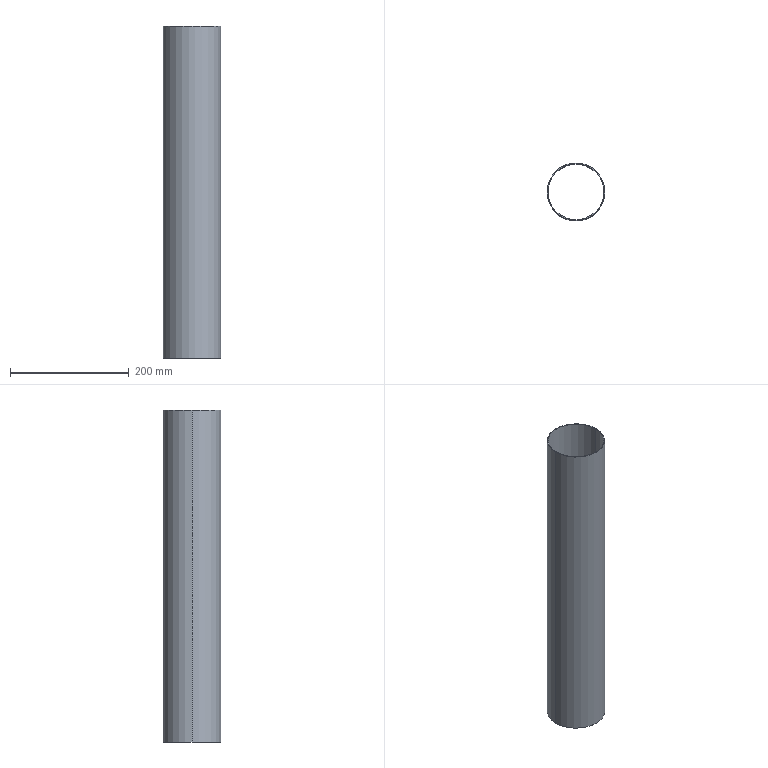Part | SolidWorks | features Extrusion 1 | 1 solid | 6 faces | box 97 x 97 x 558.5 mm | volume 201706 mm3 | cylinder 4 | plane 2 | commonest cylinder face diameters 94.6 x2 97 x2
STEP:
#1=CARTESIAN_POINT('',(-47.3,0.,558.5));
#2=VERTEX_POINT('',#1);
#3=CARTESIAN_POINT('',(47.3,0.,558.5));
#4=VERTEX_POINT('',#3);
#5=CARTESIAN_POINT('',(0.,0.,558.5));
#6=DIRECTION('',(0.,0.,1.));
#7=DIRECTION('',(1.,0.,0.));
#8=AXIS2_PLACEMENT_3D('',#5,#6,#7);
#9=CIRCLE('',#8,47.3);
#10=EDGE_CURVE('',#2,#4,#9,.T.);
#11=ORIENTED_EDGE('',*,*,#10,.T.);
#12=CARTESIAN_POINT('',(47.3,0.,0.));
#13=VERTEX_POINT('',#12);
#14=CARTESIAN_POINT('',(47.3,0.,558.5));
#15=DIRECTION('',(0.,0.,-1.));
#16=VECTOR('',#15,1000.);
#17=LINE('',#14,#16);
#18=EDGE_CURVE('',#4,#13,#17,.T.);
#19=ORIENTED_EDGE('',*,*,#18,.T.);
#20=CARTESIAN_POINT('',(-47.3,0.,0.));
#21=VERTEX_POINT('',#20);
#22=CARTESIAN_POINT('',(0.,0.,0.));
#23=DIRECTION('',(0.,0.,1.));
#24=DIRECTION('',(1.,0.,0.));
#25=AXIS2_PLACEMENT_3D('',#22,#23,#24);
#26=CIRCLE('',#25,47.3);
#27=EDGE_CURVE('',#21,#13,#26,.T.);
#28=ORIENTED_EDGE('',*,*,#27,.F.);
#29=CARTESIAN_POINT('',(-47.3,0.,558.5));
#30=DIRECTION('',(0.,0.,-1.));
#31=VECTOR('',#30,1000.);
#32=LINE('',#29,#31);
#33=EDGE_CURVE('',#2,#21,#32,.T.);
#34=ORIENTED_EDGE('',*,*,#33,.F.);
#35=EDGE_LOOP('',(#11,#19,#28,#34));
#36=FACE_OUTER_BOUND('',#35,.T.);
#37=CARTESIAN_POINT('',(0.,0.,558.5));
#38=DIRECTION('',(0.,0.,-1.));
#39=DIRECTION('',(-1.,0.,0.));
#40=AXIS2_PLACEMENT_3D('',#37,#38,#39);
#41=CYLINDRICAL_SURFACE('',#40,47.3);
#42=ADVANCED_FACE('',(#36),#41,.F.);
#43=CARTESIAN_POINT('',(48.5,0.,558.5));
#44=VERTEX_POINT('',#43);
#45=CARTESIAN_POINT('',(-48.5,0.,558.5));
#46=VERTEX_POINT('',#45);
#47=CARTESIAN_POINT('',(0.,0.,558.5));
#48=DIRECTION('',(0.,0.,1.));
#49=DIRECTION('',(1.,0.,0.));
#50=AXIS2_PLACEMENT_3D('',#47,#48,#49);
#51=CIRCLE('',#50,48.5);
#52=EDGE_CURVE('',#44,#46,#51,.T.);
#53=ORIENTED_EDGE('',*,*,#52,.F.);
#54=CARTESIAN_POINT('',(48.5,0.,0.));
#55=VERTEX_POINT('',#54);
#56=CARTESIAN_POINT('',(48.5,0.,558.5));
#57=DIRECTION('',(0.,0.,-1.));
#58=VECTOR('',#57,1000.);
#59=LINE('',#56,#58);
#60=EDGE_CURVE('',#44,#55,#59,.T.);
#61=ORIENTED_EDGE('',*,*,#60,.T.);
#62=CARTESIAN_POINT('',(-48.5,0.,0.));
#63=VERTEX_POINT('',#62);
#64=CARTESIAN_POINT('',(0.,0.,0.));
#65=DIRECTION('',(0.,0.,1.));
#66=DIRECTION('',(1.,0.,0.));
#67=AXIS2_PLACEMENT_3D('',#64,#65,#66);
#68=CIRCLE('',#67,48.5);
#69=EDGE_CURVE('',#55,#63,#68,.T.);
#70=ORIENTED_EDGE('',*,*,#69,.T.);
#71=CARTESIAN_POINT('',(-48.5,0.,558.5));
#72=DIRECTION('',(0.,0.,-1.));
#73=VECTOR('',#72,1000.);
#74=LINE('',#71,#73);
#75=EDGE_CURVE('',#46,#63,#74,.T.);
#76=ORIENTED_EDGE('',*,*,#75,.F.);
#77=EDGE_LOOP('',(#53,#61,#70,#76));
#78=FACE_OUTER_BOUND('',#77,.T.);
#79=CARTESIAN_POINT('',(0.,0.,558.5));
#80=DIRECTION('',(0.,0.,-1.));
#81=DIRECTION('',(-1.,0.,0.));
#82=AXIS2_PLACEMENT_3D('',#79,#80,#81);
#83=CYLINDRICAL_SURFACE('',#82,48.5);
#84=ADVANCED_FACE('',(#78),#83,.T.);
#85=CARTESIAN_POINT('',(0.,0.,558.5));
#86=DIRECTION('',(0.,0.,1.));
#87=DIRECTION('',(1.,0.,0.));
#88=AXIS2_PLACEMENT_3D('',#85,#86,#87);
#89=CIRCLE('',#88,48.5);
#90=EDGE_CURVE('',#46,#44,#89,.T.);
#91=ORIENTED_EDGE('',*,*,#90,.T.);
#92=ORIENTED_EDGE('',*,*,#52,.T.);
#93=EDGE_LOOP('',(#91,#92));
#94=FACE_OUTER_BOUND('',#93,.T.);
#95=ORIENTED_EDGE('',*,*,#10,.F.);
#96=CARTESIAN_POINT('',(0.,0.,558.5));
#97=DIRECTION('',(0.,0.,1.));
#98=DIRECTION('',(1.,0.,0.));
#99=AXIS2_PLACEMENT_3D('',#96,#97,#98);
#100=CIRCLE('',#99,47.3);
#101=EDGE_CURVE('',#4,#2,#100,.T.);
#102=ORIENTED_EDGE('',*,*,#101,.F.);
#103=EDGE_LOOP('',(#95,#102));
#104=FACE_BOUND('',#103,.T.);
#105=CARTESIAN_POINT('',(0.,0.,558.5));
#106=DIRECTION('',(0.,0.,1.));
#107=DIRECTION('',(1.,0.,0.));
#108=AXIS2_PLACEMENT_3D('',#105,#106,#107);
#109=PLANE('',#108);
#110=ADVANCED_FACE('',(#94,#104),#109,.T.);
#111=CARTESIAN_POINT('',(0.,0.,0.));
#112=DIRECTION('',(0.,0.,1.));
#113=DIRECTION('',(1.,0.,0.));
#114=AXIS2_PLACEMENT_3D('',#111,#112,#113);
#115=CIRCLE('',#114,48.5);
#116=EDGE_CURVE('',#63,#55,#115,.T.);
#117=ORIENTED_EDGE('',*,*,#116,.F.);
#118=ORIENTED_EDGE('',*,*,#69,.F.);
#119=EDGE_LOOP('',(#117,#118));
#120=FACE_OUTER_BOUND('',#119,.T.);
#121=ORIENTED_EDGE('',*,*,#27,.T.);
#122=CARTESIAN_POINT('',(0.,0.,0.));
#123=DIRECTION('',(0.,0.,1.));
#124=DIRECTION('',(1.,0.,0.));
#125=AXIS2_PLACEMENT_3D('',#122,#123,#124);
#126=CIRCLE('',#125,47.3);
#127=EDGE_CURVE('',#13,#21,#126,.T.);
#128=ORIENTED_EDGE('',*,*,#127,.T.);
#129=EDGE_LOOP('',(#121,#128));
#130=FACE_BOUND('',#129,.T.);
#131=CARTESIAN_POINT('',(0.,0.,0.));
#132=DIRECTION('',(0.,0.,1.));
#133=DIRECTION('',(1.,0.,0.));
#134=AXIS2_PLACEMENT_3D('',#131,#132,#133);
#135=PLANE('',#134);
#136=ADVANCED_FACE('',(#120,#130),#135,.F.);
#137=ORIENTED_EDGE('',*,*,#60,.F.);
#138=ORIENTED_EDGE('',*,*,#90,.F.);
#139=ORIENTED_EDGE('',*,*,#75,.T.);
#140=ORIENTED_EDGE('',*,*,#116,.T.);
#141=EDGE_LOOP('',(#137,#138,#139,#140));
#142=FACE_OUTER_BOUND('',#141,.T.);
#143=CARTESIAN_POINT('',(0.,0.,558.5));
#144=DIRECTION('',(0.,0.,-1.));
#145=DIRECTION('',(-1.,0.,0.));
#146=AXIS2_PLACEMENT_3D('',#143,#144,#145);
#147=CYLINDRICAL_SURFACE('',#146,48.5);
#148=ADVANCED_FACE('',(#142),#147,.T.);
#149=ORIENTED_EDGE('',*,*,#18,.F.);
#150=ORIENTED_EDGE('',*,*,#101,.T.);
#151=ORIENTED_EDGE('',*,*,#33,.T.);
#152=ORIENTED_EDGE('',*,*,#127,.F.);
#153=EDGE_LOOP('',(#149,#150,#151,#152));
#154=FACE_OUTER_BOUND('',#153,.T.);
#155=CARTESIAN_POINT('',(0.,0.,558.5));
#156=DIRECTION('',(0.,0.,-1.));
#157=DIRECTION('',(-1.,0.,0.));
#158=AXIS2_PLACEMENT_3D('',#155,#156,#157);
#159=CYLINDRICAL_SURFACE('',#158,47.3);
#160=ADVANCED_FACE('',(#154),#159,.F.);
#161=CLOSED_SHELL('',(#42,#84,#110,#136,#148,#160));
#162=MANIFOLD_SOLID_BREP('',#161);
#163=CARTESIAN_POINT('',(0.,0.,0.));
#164=DIRECTION('',(0.,0.,1.));
#165=DIRECTION('',(1.,0.,0.));
#166=AXIS2_PLACEMENT_3D('',#163,#164,#165);
#167=(LENGTH_UNIT()NAMED_UNIT(*)SI_UNIT(.MILLI.,.METRE.));
#168=UNCERTAINTY_MEASURE_WITH_UNIT(LENGTH_MEASURE(0.00001),#167,'','');
#169=(NAMED_UNIT(*)PLANE_ANGLE_UNIT()SI_UNIT($,.RADIAN.));
#170=(NAMED_UNIT(*)SI_UNIT($,.STERADIAN.)SOLID_ANGLE_UNIT());
#171=(GEOMETRIC_REPRESENTATION_CONTEXT(3)GLOBAL_UNCERTAINTY_ASSIGNED_CONTEXT((#168))GLOBAL_UNIT_ASSIGNED_CONTEXT((#167,#169,#170))REPRESENTATION_CONTEXT('',''));
#172=ADVANCED_BREP_SHAPE_REPRESENTATION('',(#162,#166),#171);